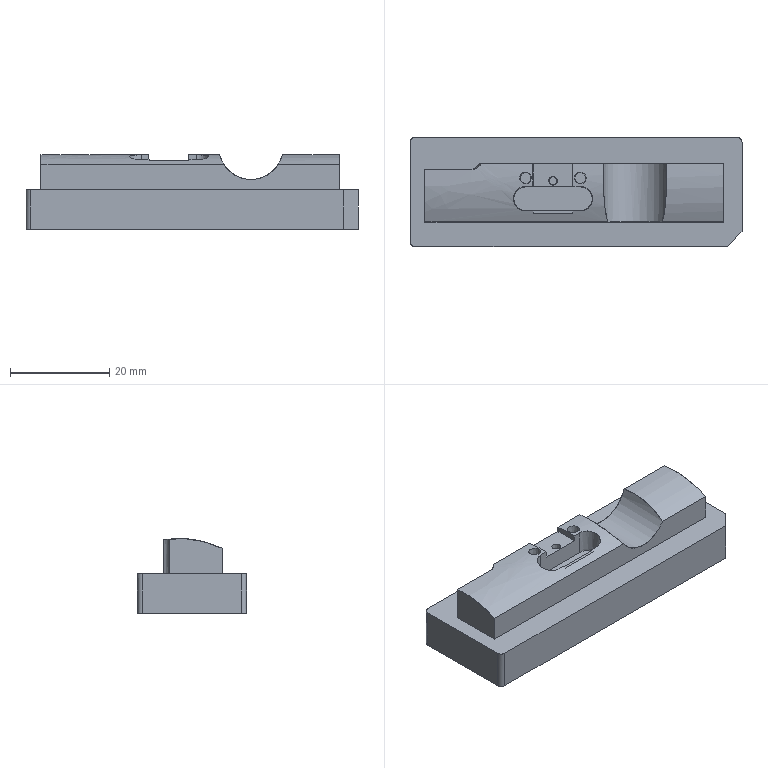NC program | PowerMill | posted with a generic post | part box 67 x 22 x 15.086 mm
Lines 17236 to 18041 of 148586:
N17333 M6
N17334 S22000 M03
N17335 G00 G90 X0.0 Y0.0
N17336 G43 Z9.7955 H27
N17337
N17338 G05 P10000 R4
N17339 X-9.6802 Y2.4709
N17340 Z0.9558
N17341 G01 Z-0.2442 F1200.0
N17342 X-9.6472 Y2.4136 Z-0.2453
N17343 X-9.623 Y2.2768 Z-0.2478
N17344 X-9.702 Y2.1939 Z-0.2498
N17345 X-9.785 Y2.1344 Z-0.2515
N17346 X-10.0186 Y2.0396 Z-0.2559
N17347 X-10.2499 Y2.0219 Z-0.26
N17348 X-10.4817 Y2.0868 Z-0.2642
N17349 X-10.5236 Y2.1139 Z-0.2651
N17350 X-10.7149 Y2.2376 Z-0.269
N17351 X-10.8641 Y2.4271 Z-0.2732
N17352 X-10.9466 Y2.6633 Z-0.2776
N17353 Y2.9354 Z-0.2824
N17354 Y2.9362
N17355 X-10.7048 Y3.0242 Z-0.2869
N17356 X-10.3749 Z-0.2926
N17357 X-10.0649 Y2.9114 Z-0.2984
N17358 X-9.8121 Y2.6993 Z-0.3041
N17359 X-9.6472 Y2.4136 Z-0.3099
N17360 X-9.623 Y2.2768 Z-0.3123
N17361 X-9.702 Y2.1939 Z-0.3143
N17362 X-9.785 Y2.1344 Z-0.3161
N17363 X-10.0186 Y2.0396 Z-0.3205
N17364 X-10.2499 Y2.0219 Z-0.3245
N17365 X-10.4817 Y2.0868 Z-0.3287
N17366 X-10.5236 Y2.1139 Z-0.3296
N17367 X-10.7149 Y2.2376 Z-0.3336
N17368 X-10.8641 Y2.4271 Z-0.3378
N17369 X-10.9466 Y2.6633 Z-0.3422
N17370 Y2.9354 Z-0.3469
N17371 Y2.9362
N17372 X-10.7048 Y3.0242 Z-0.3514
N17373 X-10.3749 Z-0.3572
N17374 X-10.0649 Y2.9114 Z-0.3629
N17375 X-9.8121 Y2.6993 Z-0.3687
N17376 X-9.6472 Y2.4136 Z-0.3745
N17377 X-9.623 Y2.2768 Z-0.3769
N17378 X-9.702 Y2.1939 Z-0.3789
N17379 X-9.785 Y2.1344 Z-0.3807
N17380 X-10.0186 Y2.0396 Z-0.3851
N17381 X-10.2499 Y2.0219 Z-0.3891
N17382 X-10.4817 Y2.0868 Z-0.3933
N17383 X-10.5236 Y2.1139 Z-0.3942
N17384 X-10.5399 Y2.0887
N17385 X-10.3183 Y2.5042 F2000.0
N17386 G03 X-9.8872 Y2.7628 I0.138 J0.2586
N17387 G03 X-10.4734 I-0.2931 J0.0
N17388 G03 X-10.3183 Y2.5042 I0.2931 J0.0
N17389 G01 X-10.5399 Y2.0887
N17390 X-10.4941 Y2.0591
N17391 X-10.2529 Y1.9915
N17392 X-10.0116 Y2.0101
N17393 X-9.7704 Y2.1079
N17394 X-9.6822 Y2.1712
N17395 X-9.5292 Y2.3319
N17396 X-9.3952 Y2.6537
N17397 X-9.3823 Y2.8949
N17398 X-9.4532 Y3.1362
N17399 X-9.6219 Y3.3774
N17400 X-9.7704 Y3.4873
N17401 X-9.9947 Y3.5797
N17402 X-10.0055 Y3.5828
N17403 X-10.0167 Y3.5834
N17404 X-10.223 Y3.6009
N17405 X-10.4941 Y3.5409
N17406 X-10.7354 Y3.3833
N17407 X-10.8391 Y3.2661
N17408 X-10.9726 Y2.9552
N17409 X-10.9756 Y2.9455
N17410 X-10.9766 Y2.9354
N17411 Y2.6582
N17412 X-10.8908 Y2.4124
N17413 X-10.7354 Y2.2151
N17414 X-10.5399 Y2.0887
N17415 X-9.8719 Y2.2967 Z-0.2934
N17416 X-9.9091 Y2.0857 Z-0.2971 F1200.0
N17417 X-10.0183 Y2.0418 Z-0.2992
N17418 X-10.25 Y2.0274 Z-0.3032
N17419 X-10.4819 Y2.0878 Z-0.3074
N17420 X-10.7149 Y2.2386 Z-0.3122
N17421 X-10.794 Y2.3394 Z-0.3145
N17422 X-10.8629 Y2.4271 Z-0.3164
N17423 X-10.9466 Y2.6664 Z-0.3208
N17424 Y2.936 Z-0.3255
N17425 X-10.9405 Y2.9538 Z-0.3259
N17426 X-10.8138 Y3.249 Z-0.3315
N17427 X-10.8071 Y3.2564 Z-0.3317
N17428 X-10.6527 Z-0.3343
N17429 X-10.3426 Y3.1436 Z-0.3401
N17430 X-10.0899 Y2.9315 Z-0.3459
N17431 X-9.9249 Y2.6458 Z-0.3516
N17432 X-9.8676 Y2.3209 Z-0.3574
N17433 X-9.9091 Y2.0857 Z-0.3615
N17434 X-10.0183 Y2.0418 Z-0.3636
N17435 X-10.25 Y2.0274 Z-0.3677
N17436 X-10.4819 Y2.0878 Z-0.3718
N17437 X-10.7149 Y2.2386 Z-0.3767
N17438 X-10.794 Y2.3394 Z-0.3789
N17439 X-10.8629 Y2.4271 Z-0.3809
N17440 X-10.9466 Y2.6664 Z-0.3853
N17441 Y2.936 Z-0.39
N17442 X-10.9405 Y2.9538 Z-0.3903
N17443 X-10.8138 Y3.249 Z-0.3959
N17444 X-10.8071 Y3.2564 Z-0.3961
N17445 X-10.6527 Z-0.3988
N17446 X-10.3426 Y3.1436 Z-0.4046
N17447 X-10.0899 Y2.9315 Z-0.4103
N17448 X-9.9249 Y2.6458 Z-0.4161
N17449 X-9.8676 Y2.3209 Z-0.4218
N17450 X-9.9091 Y2.0857 Z-0.426
N17451 X-10.0183 Y2.0418 Z-0.428
N17452 X-10.25 Y2.0274 Z-0.4321
N17453 X-10.4819 Y2.0878 Z-0.4363
N17454 X-10.7149 Y2.2386 Z-0.4411
N17455 X-10.794 Y2.3394 Z-0.4434
N17456 X-10.8176 Y2.3209
N17457 X-10.4382 Y2.6054 F2000.0
N17458 G03 X-9.9166 Y2.7793 I0.2318 J0.1739
N17459 G03 X-10.4962 I-0.2898 J0.0
N17460 G01 X-10.4813 Y2.6876
N17461 X-10.4382 Y2.6054
N17462 X-10.8176 Y2.3209
N17463 X-10.7354 Y2.2161
N17464 X-10.4941 Y2.06
N17465 X-10.2529 Y1.9971
N17466 X-10.0116 Y2.0122
N17467 X-9.7704 Y2.1091
N17468 X-9.6837 Y2.1712
N17469 X-9.6805 Y2.1745
N17470 X-9.5292 Y2.3319
N17471 X-9.3961 Y2.6537
N17472 X-9.3839 Y2.8949
N17473 X-9.454 Y3.1362
N17474 X-9.6234 Y3.3774
N17475 X-9.7704 Y3.4862
N17476 X-10.0068 Y3.583
N17477 X-10.0117 Y3.5835
N17478 X-10.0167 Y3.5834
N17479 X-10.0952 Y3.5901
N17480 X-10.2339 Y3.5986
N17481 X-10.4355 Y3.5539
N17482 X-10.4941 Y3.5392
N17483 X-10.7354 Y3.3817
N17484 X-10.8385 Y3.2663
N17485 X-10.8406 Y3.2625
N17486 X-10.9686 Y2.9646
N17487 X-10.9762 Y2.9421
N17488 X-10.9765 Y2.9399
N17489 X-10.9766 Y2.9377
N17490 Y2.6613
N17491 X-10.8895 Y2.4124
N17492 X-10.8176 Y2.3209
N17493 X-9.6903 Y2.468 Z-0.3425
N17494 X-9.6676 Y2.4287 Z-0.3433 F1200.0
N17495 X-9.6383 Y2.2625 Z-0.3463
N17496 X-9.7035 Y2.1953 Z-0.3479
N17497 X-9.7048 Y2.194 Z-0.348
N17498 X-9.7849 Y2.1368 Z-0.3497
N17499 X-10.0182 Y2.0439 Z-0.3541
N17500 X-10.25 Y2.0317 Z-0.3581
N17501 X-10.4821 Y2.0888 Z-0.3623
N17502 X-10.544 Y2.1289 Z-0.3636
N17503 X-10.7149 Y2.2396 Z-0.3671
N17504 X-10.8616 Y2.427 Z-0.3713
N17505 X-10.9466 Y2.6756 Z-0.3759
N17506 Y2.9301 Z-0.3803
N17507 X-10.9359 Y2.9627 Z-0.3809
N17508 X-10.7253 Y3.0393 Z-0.3848
N17509 X-10.3954 Z-0.3906
N17510 X-10.0853 Y2.9265 Z-0.3963
N17511 X-9.8326 Y2.7144 Z-0.4021
N17512 X-9.6676 Y2.4287 Z-0.4078
N17513 X-9.6383 Y2.2625 Z-0.4108
N17514 X-9.7035 Y2.1953 Z-0.4124
N17515 X-9.7048 Y2.194
N17516 X-9.7849 Y2.1368 Z-0.4142
N17517 X-10.0182 Y2.0439 Z-0.4185
N17518 X-10.25 Y2.0317 Z-0.4226
N17519 X-10.4821 Y2.0888 Z-0.4268
N17520 X-10.544 Y2.1289 Z-0.4281
N17521 X-10.7149 Y2.2396 Z-0.4316
N17522 X-10.8616 Y2.427 Z-0.4358
N17523 X-10.9466 Y2.6756 Z-0.4403
N17524 Y2.9301 Z-0.4448
N17525 X-10.9359 Y2.9627 Z-0.4454
N17526 X-10.7253 Y3.0393 Z-0.4493
N17527 X-10.3954 Z-0.4551
N17528 X-10.0853 Y2.9265 Z-0.4608
N17529 X-9.8326 Y2.7144 Z-0.4666
N17530 X-9.6676 Y2.4287 Z-0.4723
N17531 X-9.6383 Y2.2625 Z-0.4753
N17532 X-9.7035 Y2.1953 Z-0.4769
N17533 X-9.7048 Y2.194
N17534 X-9.7849 Y2.1368 Z-0.4787
N17535 X-10.0182 Y2.0439 Z-0.483
N17536 X-10.25 Y2.0317 Z-0.4871
N17537 X-10.4821 Y2.0888 Z-0.4913
N17538 X-10.544 Y2.1289 Z-0.4925
N17539 X-10.5603 Y2.1037
N17540 X-10.342 Y2.513 F2000.0
N17541 G03 X-9.9124 Y2.7708 I0.1375 J0.2578
N17542 G03 X-10.4967 I-0.2921 J0.0
N17543 G03 X-10.342 Y2.513 I0.2922 J0.0
N17544 G01 X-10.5603 Y2.1037
N17545 X-10.4941 Y2.0608
N17546 X-10.2529 Y2.0015
N17547 X-10.0116 Y2.0142
N17548 X-9.7704 Y2.1103
N17549 X-9.6851 Y2.1712
N17550 X-9.682 Y2.1744
N17551 X-9.5292 Y2.3319
N17552 X-9.397 Y2.6537
N17553 X-9.3849 Y2.8949
N17554 X-9.4548 Y3.1362
N17555 X-9.6248 Y3.3774
N17556 X-9.7704 Y3.4852
N17557 X-10.0116 Y3.5833
N17558 X-10.0151 Y3.5835
N17559 X-10.0159
N17560 X-10.0167
N17561 X-10.0233 Y3.584
N17562 X-10.2409 Y3.5971
N17563 X-10.3721 Y3.568
N17564 X-10.4941 Y3.5376
N17565 X-10.7354 Y3.3804
N17566 X-10.8373 Y3.266
N17567 X-10.8454 Y3.2515
N17568 X-10.9607 Y2.983
N17569 X-10.9766 Y2.935
N17570 Y2.6706
N17571 X-10.8883 Y2.4124
N17572 X-10.7354 Y2.2172
N17573 X-10.5603 Y2.1037
N17574 X-10.7679 Y2.8597 Z-0.3917
N17575 X-10.9126 Y2.9812 Z-0.395 F1200.0
N17576 X-10.922 Y2.9974 Z-0.3954
N17577 X-10.8227 Y3.2285 Z-0.3997
N17578 X-10.8115 Y3.2482 Z-0.4001
N17579 X-10.7156 Y3.3562 Z-0.4027
N17580 X-10.482 Y3.5084 Z-0.4075
N17581 X-10.2996 Y3.5534 Z-0.4108
N17582 X-10.2456 Y3.5654 Z-0.4118
N17583 X-10.1867 Y3.5619 Z-0.4128
N17584 X-10.0183 Y3.552 Z-0.4157
N17585 X-9.7852 Y3.4578 Z-0.4201
N17586 X-9.6479 Y3.3562 Z-0.4231
N17587 X-9.4832 Y3.123 Z-0.4281
N17588 X-9.4472 Y2.9985 Z-0.4304
N17589 X-9.4572 Y2.9812 Z-0.4307
N17590 X-9.7099 Y2.7691 Z-0.4365
N17591 X-10.0199 Y2.6563 Z-0.4422
N17592 X-10.3499 Z-0.448
N17593 X-10.6599 Y2.7691 Z-0.4537
N17594 X-10.9126 Y2.9812 Z-0.4595
N17595 X-10.922 Y2.9974 Z-0.4598
N17596 X-10.8227 Y3.2285 Z-0.4642
N17597 X-10.8115 Y3.2482 Z-0.4646
N17598 X-10.7156 Y3.3562 Z-0.4671
N17599 X-10.482 Y3.5084 Z-0.472
N17600 X-10.2996 Y3.5534 Z-0.4753
N17601 X-10.2456 Y3.5654 Z-0.4762
N17602 X-10.1867 Y3.5619 Z-0.4773
N17603 X-10.0183 Y3.552 Z-0.4802
N17604 X-9.7852 Y3.4578 Z-0.4846
N17605 X-9.6479 Y3.3562 Z-0.4876
N17606 X-9.4832 Y3.123 Z-0.4926
N17607 X-9.4472 Y2.9985 Z-0.4948
N17608 X-9.4572 Y2.9812 Z-0.4952
N17609 X-9.7099 Y2.7691 Z-0.5009
N17610 X-10.0199 Y2.6563 Z-0.5067
N17611 X-10.3499 Z-0.5124
N17612 X-10.6599 Y2.7691 Z-0.5182
N17613 X-10.9126 Y2.9812 Z-0.524
N17614 X-10.922 Y2.9974 Z-0.5243
N17615 X-10.8227 Y3.2285 Z-0.5287
N17616 X-10.8115 Y3.2482 Z-0.5291
N17617 X-10.7156 Y3.3562 Z-0.5316
N17618 X-10.482 Y3.5084 Z-0.5365
N17619 X-10.2996 Y3.5534 Z-0.5397
N17620 X-10.2456 Y3.5654 Z-0.5407
N17621 X-10.1867 Y3.5619 Z-0.5417
N17622 X-10.1849 Y3.5918
N17623 Y3.1341 F2000.0
N17624 G03 X-10.4808 Y2.8383 I0.0 J-0.2958
N17625 G03 X-9.889 I0.2959 J0.0
N17626 G03 X-10.1849 Y3.1341 I-0.2959 J0.0
N17627 G01 Y3.5918
N17628 X-10.248 Y3.5956
N17629 X-10.3065 Y3.5826
N17630 X-10.4941 Y3.5363
N17631 X-10.7354 Y3.3792
N17632 X-10.836 Y3.2658
N17633 X-10.8496 Y3.2419
N17634 X-10.9542 Y2.9984
N17635 X-10.9766 Y2.9287
N17636 Y2.6799
N17637 X-10.8871 Y2.4124
N17638 X-10.7354 Y2.2183
N17639 X-10.4941 Y2.0617
N17640 X-10.2529 Y2.0025
N17641 X-10.0116 Y2.0159
N17642 X-9.7704 Y2.1115
N17643 X-9.6866 Y2.1712
N17644 X-9.6834 Y2.1745
N17645 X-9.5292 Y2.3334
N17646 X-9.398 Y2.6537
N17647 X-9.386 Y2.8949
N17648 X-9.4558 Y3.1362
N17649 X-9.6262 Y3.3774
N17650 X-9.7704 Y3.4842
N17651 X-10.0116 Y3.5817
N17652 X-10.1849 Y3.5918
N17653 X-10.3126 Y3.3613 Z-0.4409
N17654 X-10.1975 Y3.5607 Z-0.4449 F1200.0
N17655 X-10.0183 Y3.5503 Z-0.4481
N17656 X-9.7852 Y3.4567 Z-0.4525
N17657 X-9.6493 Y3.3562 Z-0.4554
N17658 X-9.4841 Y3.123 Z-0.4604
N17659 X-9.454 Y3.0189 Z-0.4623
N17660 X-9.4172 Y2.8914 Z-0.4646
N17661 X-9.4286 Y2.6603 Z-0.4686
N17662 X-9.5547 Y2.3516 Z-0.4745
N17663 X-9.7064 Y2.1954 Z-0.4783
N17664 X-9.7077 Y2.1941
N17665 X-9.7632 Y2.1546 Z-0.4795
N17666 X-9.9002 Y2.2045 Z-0.482
N17667 X-10.153 Y2.4165 Z-0.4878
N17668 X-10.3179 Y2.7023 Z-0.4935
N17669 X-10.3752 Y3.0272 Z-0.4993
N17670 X-10.3179 Y3.3521 Z-0.5051
N17671 X-10.1975 Y3.5607 Z-0.5093
N17672 X-10.0183 Y3.5503 Z-0.5124
N17673 X-9.7852 Y3.4567 Z-0.5168
N17674 X-9.6493 Y3.3562 Z-0.5197
N17675 X-9.4841 Y3.123 Z-0.5247
N17676 X-9.454 Y3.0189 Z-0.5266
N17677 X-9.4172 Y2.8914 Z-0.5289
N17678 X-9.4286 Y2.6603 Z-0.533
N17679 X-9.5547 Y2.3516 Z-0.5388
N17680 X-9.7064 Y2.1954 Z-0.5426
N17681 X-9.7077 Y2.1941
N17682 X-9.7632 Y2.1546 Z-0.5438
N17683 X-9.9002 Y2.2045 Z-0.5463
N17684 X-10.153 Y2.4165 Z-0.5521
N17685 X-10.3179 Y2.7023 Z-0.5579
N17686 X-10.3752 Y3.0272 Z-0.5636
N17687 X-10.3179 Y3.3521 Z-0.5694
N17688 X-10.1975 Y3.5607 Z-0.5736
N17689 X-10.0183 Y3.5503 Z-0.5767
N17690 X-9.7852 Y3.4567 Z-0.5811
N17691 X-9.6493 Y3.3562 Z-0.584
N17692 X-9.4841 Y3.123 Z-0.589
N17693 X-9.454 Y3.0189 Z-0.5909
N17694 X-9.4252 Y3.0272
N17695 X-9.865 Y2.8989 F2000.0
N17696 G03 X-10.4404 Y2.8167 I-0.2818 J-0.0822
N17697 G03 X-9.8532 I0.2936 J0.0
N17698 G01 X-9.8562 Y2.8582
N17699 X-9.865 Y2.8989
N17700 X-9.4252 Y3.0272
N17701 X-9.4567 Y3.1362
N17702 X-9.6276 Y3.3774
N17703 X-9.7704 Y3.4831
N17704 X-10.0116 Y3.58
N17705 X-10.2529 Y3.594
N17706 X-10.4941 Y3.5351
N17707 X-10.7354 Y3.3779
N17708 X-10.8737 Y3.1859
N17709 X-10.9488 Y3.0109
N17710 X-10.9766 Y2.9224
N17711 Y2.6893
N17712 X-10.8858 Y2.4124
N17713 X-10.7354 Y2.2193
N17714 X-10.4941 Y2.0626
N17715 X-10.2529 Y2.0035
N17716 X-10.0116 Y2.0171
N17717 X-9.7704 Y2.1127
N17718 X-9.6881 Y2.1712
N17719 X-9.6849 Y2.1745
N17720 X-9.5292 Y2.3349
N17721 X-9.3989 Y2.6537
N17722 X-9.387 Y2.8949
N17723 X-9.4252 Y3.0272
N17724 X-10.7634 Y2.8626 Z-0.4901
N17725 X-10.9005 Y2.9776 Z-0.4932 F1200.0
N17726 X-10.9173 Y3.0068 Z-0.4938
N17727 X-10.9155 Y3.0126 Z-0.4939
N17728 X-10.8487 Y3.1682 Z-0.4969
N17729 X-10.7134 Y3.3553 Z-0.5009
N17730 X-10.482 Y3.5061 Z-0.5057
N17731 X-10.2501 Y3.5627 Z-0.5099
N17732 X-10.1745 Y3.5583 Z-0.5112
N17733 X-10.0183 Y3.5493 Z-0.5139
N17734 X-9.7852 Y3.4557 Z-0.5183
N17735 X-9.6507 Y3.3562 Z-0.5212
N17736 X-9.4851 Y3.123 Z-0.5262
N17737 X-9.4438 Y2.9798 Z-0.5288
N17738 X-9.445 Y2.9776 Z-0.5289
N17739 X-9.6978 Y2.7656 Z-0.5346
N17740 X-10.0078 Y2.6527 Z-0.5404
N17741 X-10.3377 Z-0.5462
N17742 X-10.6478 Y2.7656 Z-0.5519
N17743 X-10.9005 Y2.9776 Z-0.5577
N17744 X-10.9173 Y3.0068 Z-0.5583
N17745 X-10.9155 Y3.0126 Z-0.5584
N17746 X-10.8487 Y3.1682 Z-0.5613
N17747 X-10.7134 Y3.3553 Z-0.5653
N17748 X-10.482 Y3.5061 Z-0.5702
N17749 X-10.2501 Y3.5627 Z-0.5743
N17750 X-10.1745 Y3.5583 Z-0.5757
N17751 X-10.0183 Y3.5493 Z-0.5784
N17752 X-9.7852 Y3.4557 Z-0.5828
N17753 X-9.6507 Y3.3562 Z-0.5857
N17754 X-9.4851 Y3.123 Z-0.5907
N17755 X-9.4438 Y2.9798 Z-0.5933
N17756 X-9.445 Y2.9776
N17757 X-9.6978 Y2.7656 Z-0.5991
N17758 X-10.0078 Y2.6527 Z-0.6048
N17759 X-10.3377 Z-0.6106
N17760 X-10.6478 Y2.7656 Z-0.6164
N17761 X-10.9005 Y2.9776 Z-0.6221
N17762 X-10.9173 Y3.0068 Z-0.6227
N17763 X-10.9155 Y3.0126 Z-0.6228
N17764 X-10.8487 Y3.1682 Z-0.6258
N17765 X-10.7134 Y3.3553 Z-0.6298
N17766 X-10.482 Y3.5061 Z-0.6346
N17767 X-10.2501 Y3.5627 Z-0.6388
N17768 X-10.1745 Y3.5583 Z-0.6401
N17769 X-10.1728 Y3.5883
N17770 Y3.1275 F2000.0
N17771 G03 X-10.4651 Y2.8352 I0.0 J-0.2923
N17772 G03 X-9.8804 I0.2923 J0.0
N17773 G03 X-10.1728 Y3.1275 I-0.2924 J0.0
N17774 G01 Y3.5883
N17775 X-10.2529 Y3.5929
N17776 X-10.4941 Y3.534
N17777 X-10.7344 Y3.3774
N17778 X-10.875 Y3.1831
N17779 X-10.9437 Y3.023
N17780 X-10.9766 Y2.9161
N17781 Y2.6986
N17782 X-10.8847 Y2.4124
N17783 X-10.7354 Y2.2204
N17784 X-10.4941 Y2.0634
N17785 X-10.2529 Y2.0045
N17786 X-10.0116 Y2.0183
N17787 X-9.7704 Y2.1139
N17788 X-9.6895 Y2.1712
N17789 X-9.6863 Y2.1745
N17790 X-9.5292 Y2.3364
N17791 X-9.3998 Y2.6537
N17792 X-9.388 Y2.8949
N17793 X-9.4577 Y3.1362
N17794 X-9.6291 Y3.3774
N17795 X-9.7704 Y3.4821
N17796 X-10.0116 Y3.5789
N17797 X-10.1728 Y3.5883
N17798 X-9.6087 Y2.7515 Z-0.5393
N17799 X-9.4524 Y2.6203 Z-0.5429 F1200.0
N17800 X-9.449 Y2.6146 Z-0.543
N17801 X-9.5547 Y2.3547 Z-0.5479
N17802 X-9.7093 Y2.1954 Z-0.5517
N17803 X-9.7106 Y2.1941 Z-0.5518
N17804 X-9.7848 Y2.1416 Z-0.5534
N17805 X-10.0182 Y2.0491 Z-0.5577
N17806 X-10.1818 Y2.0396 Z-0.5606
N17807 X-10.2501 Y2.0357 Z-0.5618
N17808 X-10.4821 Y2.0923 Z-0.566
N17809 X-10.7148 Y2.2438 Z-0.5708
N17810 X-10.8568 Y2.4266 Z-0.5748
N17811 X-10.9142 Y2.6093 Z-0.5782
N17812 X-10.9078 Y2.6203 Z-0.5784
N17813 X-10.6551 Y2.8324 Z-0.5842
N17814 X-10.3451 Y2.9453 Z-0.5899
N17815 X-10.0151 Z-0.5957
N17816 X-9.7051 Y2.8324 Z-0.6014
N17817 X-9.4524 Y2.6203 Z-0.6072
N17818 X-9.449 Y2.6146 Z-0.6073
N17819 X-9.5547 Y2.3547 Z-0.6122
N17820 X-9.7093 Y2.1954 Z-0.6161
N17821 X-9.7106 Y2.1941
N17822 X-9.7848 Y2.1416 Z-0.6177
N17823 X-10.0182 Y2.0491 Z-0.6221
N17824 X-10.1818 Y2.0396 Z-0.6249
N17825 X-10.2501 Y2.0357 Z-0.6261
N17826 X-10.4821 Y2.0923 Z-0.6303
N17827 X-10.7148 Y2.2438 Z-0.6352
N17828 X-10.8568 Y2.4266 Z-0.6392
N17829 X-10.9142 Y2.6093 Z-0.6425
N17830 X-10.9078 Y2.6203 Z-0.6428
N17831 X-10.6551 Y2.8324 Z-0.6485
N17832 X-10.3451 Y2.9453 Z-0.6543
N17833 X-10.0151 Z-0.66
N17834 X-9.7051 Y2.8324 Z-0.6658
N17835 X-9.4524 Y2.6203 Z-0.6715
N17836 X-9.449 Y2.6146 Z-0.6717
N17837 X-9.5547 Y2.3547 Z-0.6766
N17838 X-9.7093 Y2.1954 Z-0.6804
N17839 X-9.7106 Y2.1941 Z-0.6805
N17840 X-9.7848 Y2.1416 Z-0.682
N17841 X-10.0182 Y2.0491 Z-0.6864
N17842 X-10.1818 Y2.0396 Z-0.6893
N17843 X-10.1801 Y2.0097
N17844 Y2.471 F2000.0
N17845 G03 X-9.89 Y2.7611 I0.0 J0.2901
N17846 G03 X-10.4702 I-0.2901 J0.0
N17847 G03 X-10.1801 Y2.471 I0.2901 J0.0
N17848 G01 Y2.0097
N17849 X-10.0116 Y2.0194
N17850 X-9.7704 Y2.1151
N17851 X-9.691 Y2.1712
N17852 X-9.6878 Y2.1745
N17853 X-9.5292 Y2.338
N17854 X-9.4007 Y2.6537
N17855 X-9.3891 Y2.8949
N17856 X-9.4586 Y3.1362
N17857 X-9.6305 Y3.3774
N17858 X-9.7704 Y3.481
N17859 X-10.0116 Y3.5781
N17860 X-10.2529 Y3.5919
N17861 X-10.4941 Y3.5329
N17862 X-10.7329 Y3.3774
N17863 X-10.8766 Y3.1793
N17864 X-10.9387 Y3.0349
N17865 X-10.9766 Y2.9098
N17866 Y2.7079
N17867 X-10.8838 Y2.4124
N17868 X-10.7354 Y2.2214
N17869 X-10.4941 Y2.0643
N17870 X-10.2529 Y2.0055
N17871 X-10.1801 Y2.0097
N17872 X-10.5014 Y3.2909 Z-0.5885
N17873 X-10.463 Y3.5085 Z-0.5923 F1200.0
N17874 X-10.2501 Y3.5607 Z-0.5962
N17875 X-10.0183 Y3.5475 Z-0.6002
N17876 X-9.7852 Y3.4536 Z-0.6046
N17877 X-9.6535 Y3.3561 Z-0.6074
N17878 X-9.5795 Y3.2525 Z-0.6097
N17879 X-9.4869 Y3.1229 Z-0.6124
N17880 X-9.4203 Y2.8914 Z-0.6167
N17881 X-9.4314 Y2.6602 Z-0.6207
N17882 X-9.5548 Y2.3562 Z-0.6264
N17883 X-9.576 Y2.3343 Z-0.627
N17884 X-9.72 Z-0.6295
N17885 X-10.0301 Y2.4472 Z-0.6352
N17886 X-10.2828 Y2.6593 Z-0.641
N17887 X-10.4478 Y2.945 Z-0.6467
N17888 X-10.5051 Y3.2699 Z-0.6525
N17889 X-10.463 Y3.5085 Z-0.6567
N17890 X-10.2501 Y3.5607 Z-0.6606
N17891 X-10.0183 Y3.5475 Z-0.6646
N17892 X-9.7852 Y3.4536 Z-0.669
N17893 X-9.6535 Y3.3561 Z-0.6718
N17894 X-9.5795 Y3.2525 Z-0.6741
N17895 X-9.4869 Y3.1229 Z-0.6768
N17896 X-9.4203 Y2.8914 Z-0.6811
N17897 X-9.4314 Y2.6602 Z-0.6851
N17898 X-9.5548 Y2.3562 Z-0.6908
N17899 X-9.576 Y2.3343 Z-0.6914
N17900 X-9.72 Z-0.6939
N17901 X-10.0301 Y2.4472 Z-0.6996
N17902 X-10.2828 Y2.6593 Z-0.7054
N17903 X-10.4478 Y2.945 Z-0.7111
N17904 X-10.5051 Y3.2699 Z-0.7169
N17905 X-10.463 Y3.5085 Z-0.7211
N17906 X-10.2501 Y3.5607 Z-0.7249
N17907 X-10.0183 Y3.5475 Z-0.729
N17908 X-9.7852 Y3.4536 Z-0.7334
N17909 X-9.6535 Y3.3561 Z-0.7362
N17910 X-9.5795 Y3.2525 Z-0.7385
N17911 X-9.5551 Y3.2699
N17912 X-9.9626 Y2.9643 F2000.0
N17913 G03 X-10.4373 Y2.806 I-0.211 J-0.1583
N17914 G03 X-9.9098 I0.2637 J0.0
N17915 G01 X-9.9233 Y2.8894
N17916 X-9.9626 Y2.9643
N17917 X-9.5551 Y3.2699
N17918 X-9.6319 Y3.3774
N17919 X-9.7704 Y3.48
N17920 X-10.0116 Y3.5772
N17921 X-10.2529 Y3.5909
N17922 X-10.4941 Y3.5318
N17923 X-10.7315 Y3.3774
N17924 X-10.8783 Y3.1756
N17925 X-10.934 Y3.0459
N17926 X-10.9766 Y2.9035
N17927 Y2.7173
N17928 X-10.8828 Y2.4124
N17929 X-10.7354 Y2.2225
N17930 X-10.4941 Y2.0652
N17931 X-10.2529 Y2.0065
N17932 X-10.0116 Y2.0206
N17933 X-9.7704 Y2.1163
N17934 X-9.6925 Y2.1712
N17935 X-9.6892 Y2.1746
N17936 X-9.5292 Y2.3395
N17937 X-9.4016 Y2.6537
N17938 X-9.3901 Y2.8949
N17939 X-9.4595 Y3.1362
N17940 X-9.5551 Y3.2699
N17941 X-9.9907 Y3.3451 Z-0.6377
N17942 X-9.8998 Y3.4214 Z-0.6397 F1200.0
N17943 X-9.7989 Y3.4581 Z-0.6416
N17944 X-9.7852 Y3.4525 Z-0.6419
N17945 X-9.6549 Y3.3561 Z-0.6447
N17946 X-9.4879 Y3.1229 Z-0.6497
N17947 X-9.4213 Y2.8914 Z-0.6539
N17948 X-9.4323 Y2.6602 Z-0.6579
N17949 X-9.4527 Y2.6099 Z-0.6589
N17950 X-9.5548 Y2.3577 Z-0.6636
N17951 X-9.7122 Y2.1955 Z-0.6676
N17952 X-9.7135 Y2.1941
N17953 X-9.7848 Y2.144 Z-0.6691
N17954 X-10.0182 Y2.0514 Z-0.6735
N17955 X-10.1836 Y2.0417 Z-0.6764
N17956 X-10.3176 Y2.2737 Z-0.6811
N17957 X-10.3748 Y2.5986 Z-0.6868
N17958 X-10.3176 Y2.9236 Z-0.6926
N17959 X-10.1526 Y3.2093 Z-0.6984
N17960 X-9.8998 Y3.4214 Z-0.7041
N17961 X-9.7989 Y3.4581 Z-0.706
N17962 X-9.7852 Y3.4525 Z-0.7062
N17963 X-9.6549 Y3.3561 Z-0.7091
N17964 X-9.4879 Y3.1229 Z-0.7141
N17965 X-9.4213 Y2.8914 Z-0.7183
N17966 X-9.4323 Y2.6602 Z-0.7223
N17967 X-9.4527 Y2.6099 Z-0.7233
N17968 X-9.5548 Y2.3577 Z-0.728
N17969 X-9.7122 Y2.1955 Z-0.732
N17970 X-9.7135 Y2.1941
N17971 X-9.7848 Y2.144 Z-0.7335
N17972 X-10.0182 Y2.0514 Z-0.7379
N17973 X-10.1836 Y2.0417 Z-0.7408
N17974 X-10.3176 Y2.2737 Z-0.7455
N17975 X-10.3748 Y2.5986 Z-0.7512
N17976 X-10.3176 Y2.9236 Z-0.757
N17977 X-10.1526 Y3.2093 Z-0.7627
N17978 X-9.8998 Y3.4214 Z-0.7685
N17979 X-9.7989 Y3.4581 Z-0.7704
N17980 X-9.7852 Y3.4525 Z-0.7706
N17981 X-9.6549 Y3.3561 Z-0.7735
N17982 X-9.4879 Y3.1229 Z-0.7785
N17983 X-9.4213 Y2.8914 Z-0.7827
N17984 X-9.4323 Y2.6602 Z-0.7867
N17985 X-9.4527 Y2.6099 Z-0.7877
N17986 X-9.4248 Y2.5986
N17987 X-9.8714 Y2.7289 F2000.0
N17988 X-9.8629 Y2.7686
N17989 X-9.86 Y2.8091
N17990 G03 X-10.4331 I-0.2865 J0.0
N17991 G03 X-9.8714 Y2.7289 I0.2866 J0.0
N17992 G01 X-9.4248 Y2.5986
N17993 X-9.4026 Y2.6537
N17994 X-9.3911 Y2.8949
N17995 X-9.4605 Y3.1362
N17996 X-9.6333 Y3.3774
N17997 X-9.7704 Y3.4789
N17998 X-10.0116 Y3.5763
N17999 X-10.2529 Y3.5899
N18000 X-10.4941 Y3.5306
N18001 X-10.73 Y3.3774
N18002 X-10.7389 Y3.3673
N18003 X-10.8635 Y3.196
N18004 X-10.9147 Y3.0908
N18005 X-10.934 Y3.0459
N18006 X-10.9538 Y2.9799
N18007 X-10.9766 Y2.7266
N18008 X-10.8819 Y2.4124
N18009 X-10.7354 Y2.2235
N18010 X-10.4941 Y2.0661
N18011 X-10.2529 Y2.0075
N18012 X-10.0116 Y2.0218
N18013 X-9.7704 Y2.1175
N18014 X-9.6939 Y2.1712
N18015 X-9.6907 Y2.1746
N18016 X-9.5292 Y2.341
N18017 X-9.4248 Y2.5986
N18018 X-9.9954 Y3.3423 Z-0.6868
N18019 X-9.9005 Y3.422 Z-0.689 F1200.0
N18020 X-9.8014 Y3.458 Z-0.6908
N18021 X-9.7852 Y3.4515 Z-0.6911
N18022 X-9.6563 Y3.3561 Z-0.6939
N18023 X-9.4888 Y3.1229 Z-0.699
N18024 X-9.4224 Y2.8914 Z-0.7032
N18025 X-9.4332 Y2.6602 Z-0.7072
N18026 X-9.4533 Y2.6105 Z-0.7081
N18027 X-9.5548 Y2.3592 Z-0.7129
N18028 X-9.7136 Y2.1955 Z-0.7168
N18029 X-9.715 Y2.1941 Z-0.7169
N18030 X-9.7847 Y2.1452 Z-0.7184
N18031 X-10.0182 Y2.0526 Z-0.7228
N18032 X-10.1844 Y2.0427 Z-0.7257
N18033 X-10.3182 Y2.2743 Z-0.7303
N18034 X-10.3755 Y2.5992 Z-0.7361
N18035 X-10.3182 Y2.9242 Z-0.7418
N18036 X-10.1532 Y3.2099 Z-0.7476
N18037 X-9.9005 Y3.422 Z-0.7534
N18038 X-9.8014 Y3.458 Z-0.7552
N18039 X-9.7852 Y3.4515 Z-0.7555
N18040 X-9.6563 Y3.3561 Z-0.7583
N18041 X-9.4888 Y3.1229 Z-0.7633
N18042 X-9.4224 Y2.8914 Z-0.7675
N18043 X-9.4332 Y2.6602 Z-0.7716
N18044 X-9.4533 Y2.6105 Z-0.7725
N18045 X-9.5548 Y2.3592 Z-0.7772
N18046 X-9.7136 Y2.1955 Z-0.7812
N18047 X-9.715 Y2.1941
N18048 X-9.7847 Y2.1452 Z-0.7827
N18049 X-10.0182 Y2.0526 Z-0.7871
N18050 X-10.1844 Y2.0427 Z-0.79
N18051 X-10.3182 Y2.2743 Z-0.7947
N18052 X-10.3755 Y2.5992 Z-0.8004
N18053 X-10.3182 Y2.9242 Z-0.8062
N18054 X-10.1532 Y3.2099 Z-0.8119
N18055 X-9.9005 Y3.422 Z-0.8177
N18056 X-9.8014 Y3.458 Z-0.8195
N18057 X-9.7852 Y3.4515 Z-0.8199
N18058 X-9.6563 Y3.3561 Z-0.8227
N18059 X-9.4888 Y3.1229 Z-0.8277
N18060 X-9.4224 Y2.8914 Z-0.8319
N18061 X-9.4332 Y2.6602 Z-0.8359
N18062 X-9.4533 Y2.6105 Z-0.8368
N18063 X-9.4255 Y2.5992
N18064 X-9.8723 Y2.7296 F2000.0
N18065 X-9.8637 Y2.7692
N18066 X-9.8608 Y2.8096
N18067 G03 X-10.4326 I-0.2859 J0.0
N18068 G03 X-9.8723 Y2.7296 I0.2859 J0.0
N18069 G01 X-9.4255 Y2.5992
N18070 X-9.4035 Y2.6537
N18071 X-9.3922 Y2.8949
N18072 X-9.4614 Y3.1362
N18073 X-9.6347 Y3.3774
N18074 X-9.7704 Y3.4779
N18075 X-10.0116 Y3.5754
N18076 X-10.2529 Y3.5889
N18077 X-10.4941 Y3.5295
N18078 X-10.7285 Y3.3774
N18079 X-10.7464 Y3.3571
N18080 X-10.8597 Y3.2013
N18081 X-10.9236 Y3.0703
N18082 X-10.9341 Y3.0459
N18083 X-10.9525 Y2.9842
N18084 X-10.9655 Y2.8511
N18085 X-10.976 Y2.7339
N18086 X-10.8809 Y2.4124
N18087 X-10.7354 Y2.2246
N18088 X-10.4941 Y2.0669
N18089 X-10.2529 Y2.0085
N18090 X-10.0116 Y2.0229
N18091 X-9.7704 Y2.1186
N18092 X-9.6954 Y2.1712
N18093 X-9.6921 Y2.1746
N18094 X-9.5292 Y2.3425
N18095 X-9.4255 Y2.5992
N18096 X-10.5043 Y3.2798 Z-0.736
N18097 X-10.4647 Y3.5047 Z-0.74 F1200.0
N18098 X-10.2501 Y3.5576 Z-0.7439
N18099 X-10.0183 Y3.5449 Z-0.7479
N18100 X-9.7852 Y3.4505 Z-0.7523
N18101 X-9.6577 Y3.3561 Z-0.7551
N18102 X-9.5809 Y3.2495 Z-0.7574
N18103 X-9.4897 Y3.1229 Z-0.7601
N18104 X-9.4234 Y2.8914 Z-0.7643
N18105 X-9.4341 Y2.6602 Z-0.7683
N18106 X-9.5548 Y2.3607 Z-0.774
N18107 X-9.5832 Y2.3315 Z-0.7747
N18108 X-9.7216 Z-0.7771
N18109 X-10.0316 Y2.4443 Z-0.7829
N18110 X-10.2843 Y2.6564 Z-0.7886
N18111 X-10.4493 Y2.9421 Z-0.7944
N18112 X-10.5066 Y3.267 Z-0.8001
N18113 X-10.4647 Y3.5047 Z-0.8043
N18114 X-10.2501 Y3.5576 Z-0.8082
N18115 X-10.0183 Y3.5449 Z-0.8123
N18116 X-9.7852 Y3.4505 Z-0.8166
N18117 X-9.6577 Y3.3561 Z-0.8194
N18118 X-9.5809 Y3.2495 Z-0.8217
N18119 X-9.4897 Y3.1229 Z-0.8244
N18120 X-9.4234 Y2.8914 Z-0.8286
N18121 X-9.4341 Y2.6602 Z-0.8327
N18122 X-9.5548 Y2.3607 Z-0.8383
N18123 X-9.5832 Y2.3315 Z-0.839
N18124 X-9.7216 Z-0.8414
N18125 X-10.0316 Y2.4443 Z-0.8472
N18126 X-10.2843 Y2.6564 Z-0.8529
N18127 X-10.4493 Y2.9421 Z-0.8587
N18128 X-10.5066 Y3.267 Z-0.8645
N18129 X-10.4647 Y3.5047 Z-0.8687
N18130 X-10.2501 Y3.5576 Z-0.8725
N18131 X-10.0183 Y3.5449 Z-0.8766
N18132 X-9.7852 Y3.4505 Z-0.881
N18133 X-9.6577 Y3.3561 Z-0.8837
N18134 X-9.5809 Y3.2495 Z-0.886
N18135 X-9.5566 Y3.267
N18136 X-9.9207 Y2.994 F2000.0
N18137 G03 X-10.4367 Y2.822 I-0.2293 J-0.172
N18138 G03 X-9.8633 I0.2867 J0.0